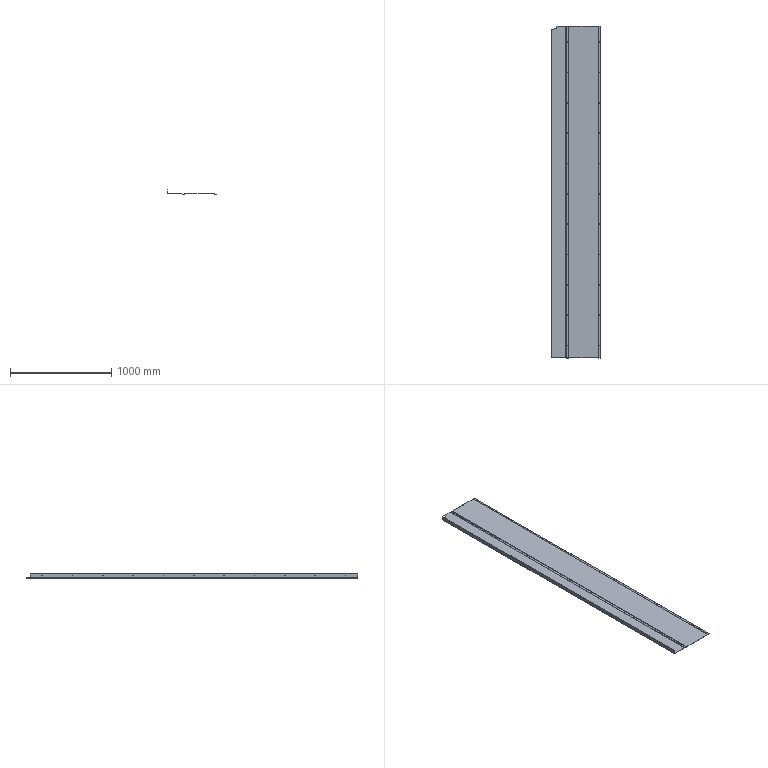Part | STEP file | TS-S86 | 1 solid | 135 faces | box 488 x 3283 x 43 mm | volume 2083173 mm3 | cylinder 83 | plane 52 | commonest cylinder face diameters 5.4 x66 0.4 x7 2.8 x7 10 x1 16 x1 18 x1